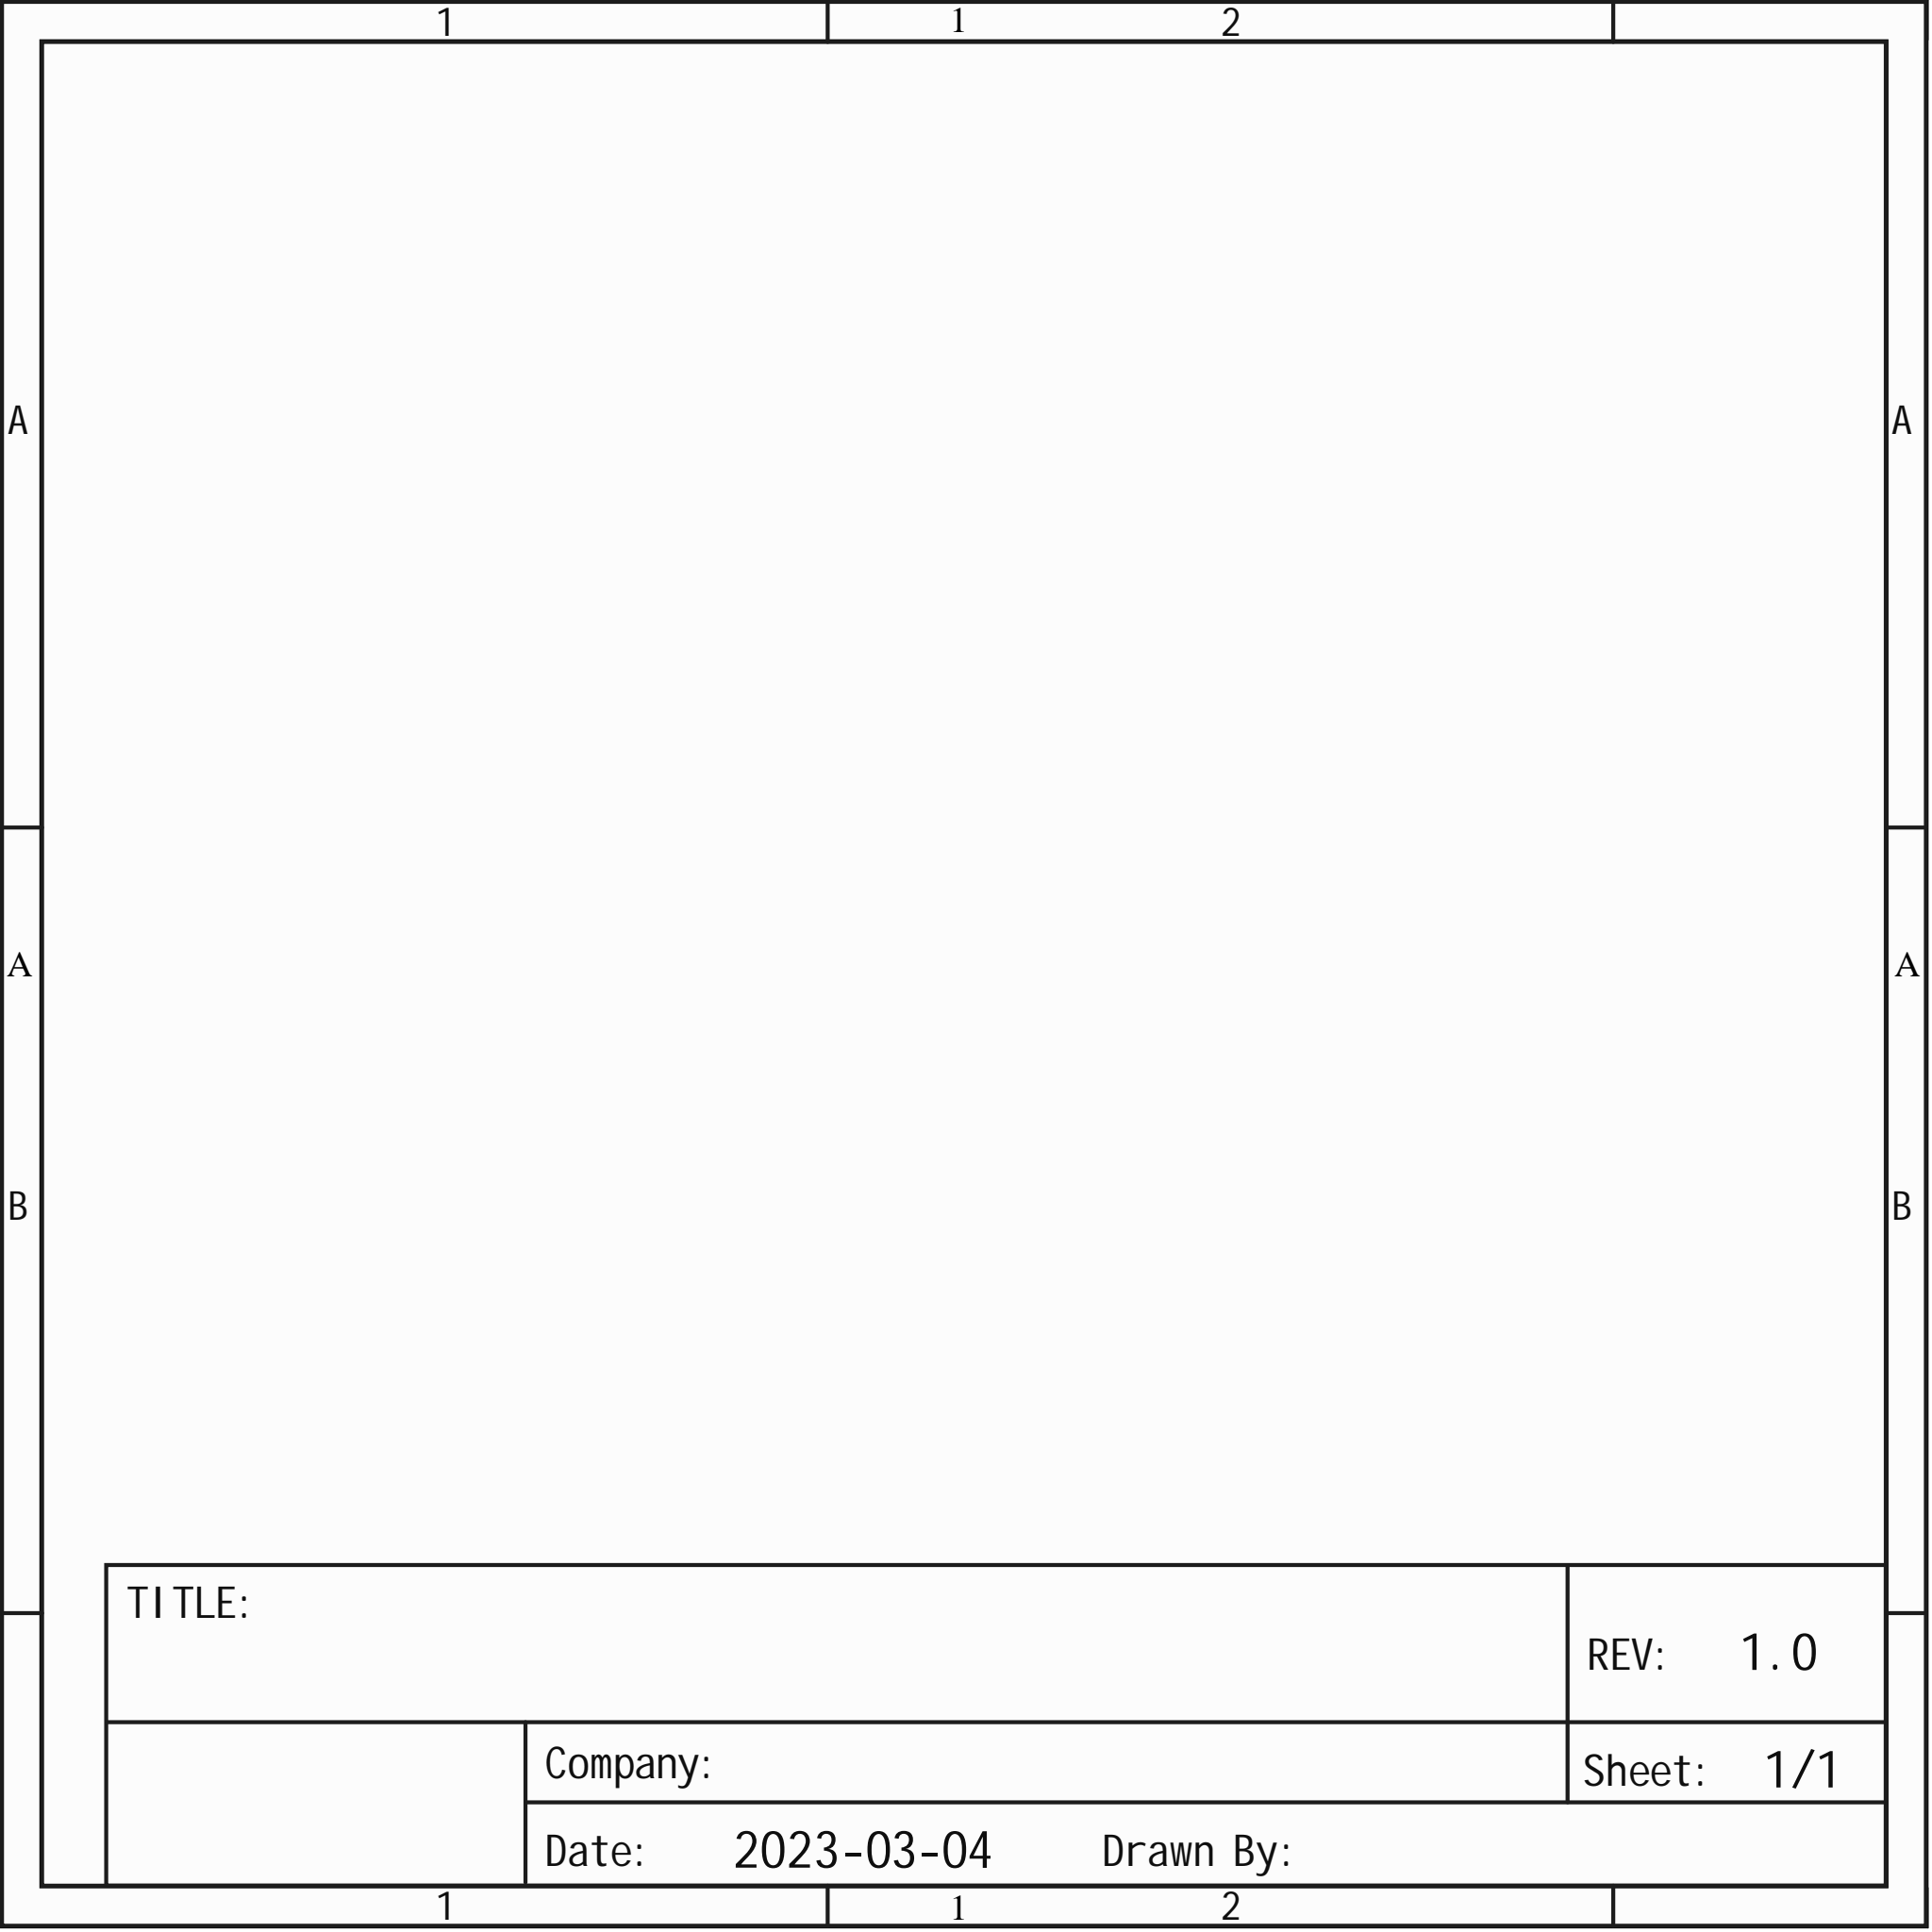Circuit board | Altium Designer | 50 parts | 48 nets
Bill of materials:
Comment,Description,Designator,Footprint,LibRef,Quantity
"33p","","C1, C2","C0805","33p","2"
"10NF","","C4","C0805","10NF","1"
"10uF","","C5, C6","CAP-TH_BD10.0-P5.00-D1.0-FD","EGS2GM100G12OTG","2"
"HC-SR04","","H2","HC-SR04","HC-SR04","1"
"HDR-M-2.54_1x8","","J1, J2, J3, J4","HDR-M-2.54_1X8","HDR-M-2.54_1x8","4"
"HDR-M-2.54_1x4","","J5","HDR-M-2.54_1X4","HDR-M-2.54_1x4","1"
"HDR-M-2.54_1x3","","J6","HDR-M-2.54_1X3","HDR-M-2.54_1x3","1"
"K2-3.6×6.1_SMD","","KEY1, KEY2, KEY3, KEY4, KEY5","KEY-SMD_2P-L6.2-W3.6-LS8.0","K2-1107ST-A4SW-06","5"
"LED-0805_R","","LED1, LED2","LED0805_RED","17-21SURC/S530-A3/TR8","2"
"204-10SDRD/S530-A3-L","","LED3, LED4, LED5, LED6, LED7, LED8","LED-TH_BD3.8-P2.54-FD","204-10SDRD/S530-A3-L","6"
"10k","","R1","R0805","10k","1"
"1.5k","","R2","R0805","1.5k","1"
"1k","","R3","R0805","1k","1"
"4.7k","","R4, R5, R6, R7, R8, R9, R10, R11","R0805","4.7k","8"
"1000","","R12, R13, R14, R15, R16, R17","R0603","1000","6"
"10kΩ","","R18, R19","RES-ADJ-TH_3296W","3296W-1-103LF","2"
"","","SCREW1, SCREW2","M2螺丝","M2螺丝","2"
"MST22D18G2 125","","SW2","SW-SMD_MST22D18G2","MST22D18G2 125","1"
"STC90C52RC-40I_C14023","","U1","DIP-40_L52.0-W13.7-P2.54-LS15.2-BL","STC90C52RC-40I","1"
"USB-Micro_1","","USB4","MICRO-USB-SMD_5P-P0.65-H-F_C10418","USB-Micro_1","1"
"11.059MHz","","X1","OSC-TH_L10.0-W4.5-P5.00","X49UD110592MSD2SC","1"
Netlist (Protel format):
[
C1
C0805
33p



]
[
C2
C0805
33p



]
[
C4
C0805
10NF



]
[
C5
CAP-TH_BD10.0-P5.00-D1.0-FD
10uF



]
[
C6
CAP-TH_BD10.0-P5.00-D1.0-FD
10uF



]
[
H2
HC-SR04
HC-SR04



]
[
J1
HDR-M-2.54_1X8
HDR-M-2.54_1x8



]
[
J2
HDR-M-2.54_1X8
HDR-M-2.54_1x8



]
[
J3
HDR-M-2.54_1X8
HDR-M-2.54_1x8



]
[
J4
HDR-M-2.54_1X8
HDR-M-2.54_1x8



]
[
J5
HDR-M-2.54_1X4
HDR-M-2.54_1x4



]
[
J6
HDR-M-2.54_1X3
HDR-M-2.54_1x3



]
[
KEY1
KEY-SMD_2P-L6.2-W3.6-LS8.0
K2-3.6×6.1_SMD



]
[
KEY2
KEY-SMD_2P-L6.2-W3.6-LS8.0
K2-3.6×6.1_SMD



]
[
KEY3
KEY-SMD_2P-L6.2-W3.6-LS8.0
K2-3.6×6.1_SMD



]
[
KEY4
KEY-SMD_2P-L6.2-W3.6-LS8.0
K2-3.6×6.1_SMD



]
[
KEY5
KEY-SMD_2P-L6.2-W3.6-LS8.0
K2-3.6×6.1_SMD



]
[
LED1
LED0805_RED
LED-0805_R



]
[
LED2
LED0805_RED
LED-0805_R



]
[
LED3
LED-TH_BD3.8-P2.54-FD
204-10SDRD/S530-A3-L



]
[
LED4
LED-TH_BD3.8-P2.54-FD
204-10SDRD/S530-A3-L



]
[
LED5
LED-TH_BD3.8-P2.54-FD
204-10SDRD/S530-A3-L



]
[
LED6
LED-TH_BD3.8-P2.54-FD
204-10SDRD/S530-A3-L



]
[
LED7
LED-TH_BD3.8-P2.54-FD
204-10SDRD/S530-A3-L



]
[
LED8
LED-TH_BD3.8-P2.54-FD
204-10SDRD/S530-A3-L



]
[
R1
R0805
10k



]
[
R2
R0805
1.5k



]
[
R3
R0805
1k



]
[
R4
R0805
4.7k



]
[
R5
R0805
4.7k



]
[
R6
R0805
4.7k



]
[
R7
R0805
4.7k



]
[
R8
R0805
4.7k



]
[
R9
R0805
4.7k



]
[
R10
R0805
4.7k



]
[
R11
R0805
4.7k



]
[
R12
R0603
1000



]
[
R13
R0603
1000



]
[
R14
R0603
1000



]
[
R15
R0603
1000



]
[
R16
R0603
1000



]
[
R17
R0603
1000



]
[
R18
RES-ADJ-TH_3296W
10kΩ



]
[
R19
RES-ADJ-TH_3296W
10kΩ



]
[
SCREW1
M2螺丝




]
[
SCREW2
M2螺丝




]
[
SW2
SW-SMD_MST22D18G2
MST22D18G2 125



]
[
U1
DIP-40_L52.0-W13.7-P2.54-LS15.2-BL
STC90C52RC-40I_C14023



]
[
USB4
MICRO-USB-SMD_5P-P0.65-H-F_C10418
USB-Micro_1



]
[
X1
OSC-TH_L10.0-W4.5-P5.00
11.0592MHz



]
(
XTAL2
C1-2
U1-18
X1-1
)
(
XTAL1
C2-2
U1-19
X1-2
)
(
TXD
J4-7
J5-3
U1-11
)
(
RXD
J4-8
J5-2
U1-10
)
(
RST
KEY2-1
U1-9
)
(
P3.5
J4-3
KEY5-2
U1-15
)
(
P3.4
J4-4
KEY1-2
U1-14
)
(
P3.3
J4-5
KEY3-2
U1-13
)
(
P3.2
J4-6
KEY4-2
U1-12
)
(
P2.7
J2-1
LED2-2
U1-28
)
(
P2.6
J2-2
U1-27
)
(
P2.5
J2-3
U1-26
)
(
P2.4
J2-4
J6-2
U1-25
)
(
P2.3
J2-5
R18-3
U1-24
)
(
P2.2
J2-6
R19-3
U1-23
)
(
P2.1
H2-2
J2-7
U1-22
)
(
P2.0
H2-3
J2-8
U1-21
)
(
P0.7
J1-8
R11-1
U1-32
)
(
P0.6
J1-7
R10-1
U1-33
)
(
P0.5
J1-6
R9-1
U1-34
)
(
P0.4
J1-5
R8-1
U1-35
)
(
P0.3
J1-4
R7-1
U1-36
)
(
P0.2
J1-3
R6-1
U1-37
)
(
P0.1
J1-2
R5-1
U1-38
)
(
P0.0
J1-1
R4-1
U1-39
)
(
NetSW2_2
SW2-2
USB4-1
)
(
NetR15_2
R15-2
R16-2
R17-2
R19-1
R19-2
)
(
NetLED8_2
LED8-2
R17-1
)
(
NetLED7_2
LED7-2
R16-1
)
(
NetLED6_2
LED6-2
R15-1
)
(
NetLED5_2
LED5-2
R14-1
)
(
NetLED4_2
LED4-2
R12-1
R12-2
R13-2
R14-2
R18-1
R18-2
)
(
NetLED3_2
LED3-2
R13-1
)
(
NetLED2_1
LED2-1
R3-1
)
(
NetLED1_1
LED1-1
R2-1
)
(
NetJ4_2
J4-2
U1-16
)
(
NetJ4_1
J4-1
U1-17
)
(
NetJ3_8
J3-8
U1-1
)
(
NetJ3_7
J3-7
U1-2
)
(
NetJ3_6
J3-6
U1-3
)
(
NetJ3_5
J3-5
U1-4
)
(
NetJ3_4
J3-4
U1-5
)
(
NetJ3_3
J3-3
U1-6
)
(
NetJ3_2
J3-2
U1-7
)
(
NetJ3_1
J3-1
U1-8
)
(
NetC5_2
C5-2
R1-2
)
(
GND
C1-1
C2-1
C4-1
C6-2
H2-4
J5-4
J6-3
KEY1-1
KEY3-1
KEY4-1
KEY5-1
LED1-2
R1-1
U1-20
USB4-5
)
(
+5V
C4-2
C5-1
C6-1
H2-1
J5-1
J6-1
KEY2-2
LED3-1
LED4-1
LED5-1
LED6-1
LED7-1
LED8-1
R2-2
R3-2
R4-2
R5-2
R6-2
R7-2
R8-2
R9-2
R10-2
R11-2
SW2-3
U1-40
)